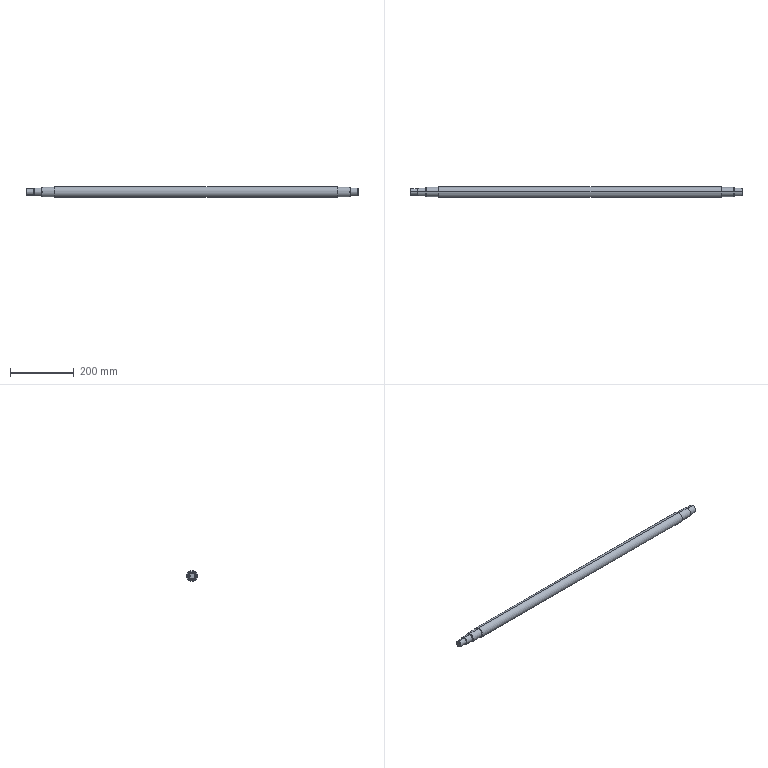Part | NX | features BREP 1 | 1 solid | 45 faces | box 1045 x 34 x 34 mm | volume 895297 mm3 | cylinder 18 | plane 17 | cone 10 | commonest cylinder face diameters 8 x4 25 x4 30 x4 6 x2 20 x2 34 x2
STEP:
#1=CARTESIAN_POINT('',(90.,0.,-17.));
#2=VERTEX_POINT('',#1);
#3=CARTESIAN_POINT('',(980.,0.,-17.));
#4=VERTEX_POINT('',#3);
#5=CARTESIAN_POINT('',(980.,0.,-17.));
#6=DIRECTION('',(-1.,0.,0.));
#7=VECTOR('',#6,1000.);
#8=LINE('',#5,#7);
#9=EDGE_CURVE('',#2,#4,#8,.F.);
#10=ORIENTED_EDGE('',*,*,#9,.T.);
#11=CARTESIAN_POINT('',(980.,0.,17.));
#12=VERTEX_POINT('',#11);
#13=CARTESIAN_POINT('',(980.,0.,0.));
#14=DIRECTION('',(-1.,0.,0.));
#15=DIRECTION('',(0.,0.,1.));
#16=AXIS2_PLACEMENT_3D('',#13,#14,#15);
#17=CIRCLE('',#16,17.);
#18=EDGE_CURVE('',#4,#12,#17,.T.);
#19=ORIENTED_EDGE('',*,*,#18,.T.);
#20=CARTESIAN_POINT('',(90.,0.,17.));
#21=VERTEX_POINT('',#20);
#22=CARTESIAN_POINT('',(980.,0.,17.));
#23=DIRECTION('',(-1.,0.,0.));
#24=VECTOR('',#23,1000.);
#25=LINE('',#22,#24);
#26=EDGE_CURVE('',#21,#12,#25,.F.);
#27=ORIENTED_EDGE('',*,*,#26,.F.);
#28=CARTESIAN_POINT('',(90.,0.,0.));
#29=DIRECTION('',(1.,0.,0.));
#30=DIRECTION('',(0.,0.,1.));
#31=AXIS2_PLACEMENT_3D('',#28,#29,#30);
#32=CIRCLE('',#31,17.);
#33=EDGE_CURVE('',#21,#2,#32,.T.);
#34=ORIENTED_EDGE('',*,*,#33,.T.);
#35=EDGE_LOOP('',(#10,#19,#27,#34));
#36=FACE_BOUND('',#35,.T.);
#37=CARTESIAN_POINT('',(980.,0.,0.));
#38=DIRECTION('',(-1.,0.,0.));
#39=DIRECTION('',(0.,0.,1.));
#40=AXIS2_PLACEMENT_3D('',#37,#38,#39);
#41=CYLINDRICAL_SURFACE('',#40,17.);
#42=ADVANCED_FACE('',(#36),#41,.T.);
#43=CARTESIAN_POINT('',(90.,0.,15.));
#44=VERTEX_POINT('',#43);
#45=CARTESIAN_POINT('',(90.,0.,-15.));
#46=VERTEX_POINT('',#45);
#47=CARTESIAN_POINT('',(90.,0.,0.));
#48=DIRECTION('',(-1.,0.,0.));
#49=DIRECTION('',(0.,0.,1.));
#50=AXIS2_PLACEMENT_3D('',#47,#48,#49);
#51=CIRCLE('',#50,15.);
#52=EDGE_CURVE('',#44,#46,#51,.T.);
#53=ORIENTED_EDGE('',*,*,#52,.F.);
#54=CARTESIAN_POINT('',(90.,0.,0.));
#55=DIRECTION('',(-1.,0.,0.));
#56=DIRECTION('',(0.,0.,1.));
#57=AXIS2_PLACEMENT_3D('',#54,#55,#56);
#58=CIRCLE('',#57,15.);
#59=EDGE_CURVE('',#46,#44,#58,.T.);
#60=ORIENTED_EDGE('',*,*,#59,.F.);
#61=EDGE_LOOP('',(#53,#60));
#62=FACE_BOUND('',#61,.T.);
#63=ORIENTED_EDGE('',*,*,#33,.F.);
#64=CARTESIAN_POINT('',(90.,0.,0.));
#65=DIRECTION('',(1.,0.,0.));
#66=DIRECTION('',(0.,0.,1.));
#67=AXIS2_PLACEMENT_3D('',#64,#65,#66);
#68=CIRCLE('',#67,17.);
#69=EDGE_CURVE('',#2,#21,#68,.T.);
#70=ORIENTED_EDGE('',*,*,#69,.F.);
#71=EDGE_LOOP('',(#63,#70));
#72=FACE_BOUND('',#71,.T.);
#73=CARTESIAN_POINT('',(90.,0.,0.));
#74=DIRECTION('',(1.,0.,0.));
#75=DIRECTION('',(0.,1.,0.));
#76=AXIS2_PLACEMENT_3D('',#73,#74,#75);
#77=PLANE('',#76);
#78=ADVANCED_FACE('',(#62,#72),#77,.F.);
#79=CARTESIAN_POINT('',(980.,0.,15.));
#80=VERTEX_POINT('',#79);
#81=CARTESIAN_POINT('',(980.,0.,-15.));
#82=VERTEX_POINT('',#81);
#83=CARTESIAN_POINT('',(980.,0.,0.));
#84=DIRECTION('',(-1.,0.,0.));
#85=DIRECTION('',(0.,0.,1.));
#86=AXIS2_PLACEMENT_3D('',#83,#84,#85);
#87=CIRCLE('',#86,15.);
#88=EDGE_CURVE('',#80,#82,#87,.T.);
#89=ORIENTED_EDGE('',*,*,#88,.T.);
#90=CARTESIAN_POINT('',(980.,0.,0.));
#91=DIRECTION('',(-1.,0.,0.));
#92=DIRECTION('',(0.,0.,1.));
#93=AXIS2_PLACEMENT_3D('',#90,#91,#92);
#94=CIRCLE('',#93,15.);
#95=EDGE_CURVE('',#82,#80,#94,.T.);
#96=ORIENTED_EDGE('',*,*,#95,.T.);
#97=EDGE_LOOP('',(#89,#96));
#98=FACE_BOUND('',#97,.T.);
#99=CARTESIAN_POINT('',(980.,0.,0.));
#100=DIRECTION('',(-1.,0.,0.));
#101=DIRECTION('',(0.,0.,1.));
#102=AXIS2_PLACEMENT_3D('',#99,#100,#101);
#103=CIRCLE('',#102,17.);
#104=EDGE_CURVE('',#12,#4,#103,.T.);
#105=ORIENTED_EDGE('',*,*,#104,.F.);
#106=ORIENTED_EDGE('',*,*,#18,.F.);
#107=EDGE_LOOP('',(#105,#106));
#108=FACE_BOUND('',#107,.T.);
#109=CARTESIAN_POINT('',(980.,0.,0.));
#110=DIRECTION('',(1.,0.,0.));
#111=DIRECTION('',(0.,1.,0.));
#112=AXIS2_PLACEMENT_3D('',#109,#110,#111);
#113=PLANE('',#112);
#114=ADVANCED_FACE('',(#98,#108),#113,.T.);
#115=CARTESIAN_POINT('',(51.,0.,-15.));
#116=VERTEX_POINT('',#115);
#117=CARTESIAN_POINT('',(90.,0.,-15.));
#118=DIRECTION('',(-1.,0.,0.));
#119=VECTOR('',#118,1000.);
#120=LINE('',#117,#119);
#121=EDGE_CURVE('',#116,#46,#120,.F.);
#122=ORIENTED_EDGE('',*,*,#121,.T.);
#123=ORIENTED_EDGE('',*,*,#59,.T.);
#124=CARTESIAN_POINT('',(51.,0.,15.));
#125=VERTEX_POINT('',#124);
#126=CARTESIAN_POINT('',(90.,0.,15.));
#127=DIRECTION('',(-1.,0.,0.));
#128=VECTOR('',#127,1000.);
#129=LINE('',#126,#128);
#130=EDGE_CURVE('',#125,#44,#129,.F.);
#131=ORIENTED_EDGE('',*,*,#130,.F.);
#132=CARTESIAN_POINT('',(51.,0.,0.));
#133=DIRECTION('',(1.,0.,0.));
#134=DIRECTION('',(0.,0.,1.));
#135=AXIS2_PLACEMENT_3D('',#132,#133,#134);
#136=CIRCLE('',#135,15.);
#137=EDGE_CURVE('',#125,#116,#136,.T.);
#138=ORIENTED_EDGE('',*,*,#137,.T.);
#139=EDGE_LOOP('',(#122,#123,#131,#138));
#140=FACE_BOUND('',#139,.T.);
#141=CARTESIAN_POINT('',(90.,0.,0.));
#142=DIRECTION('',(-1.,0.,0.));
#143=DIRECTION('',(0.,0.,1.));
#144=AXIS2_PLACEMENT_3D('',#141,#142,#143);
#145=CYLINDRICAL_SURFACE('',#144,15.);
#146=ADVANCED_FACE('',(#140),#145,.T.);
#147=CARTESIAN_POINT('',(1019.,0.,-15.));
#148=VERTEX_POINT('',#147);
#149=CARTESIAN_POINT('',(1020.,0.,-15.));
#150=DIRECTION('',(-1.,0.,0.));
#151=VECTOR('',#150,1000.);
#152=LINE('',#149,#151);
#153=EDGE_CURVE('',#82,#148,#152,.F.);
#154=ORIENTED_EDGE('',*,*,#153,.T.);
#155=CARTESIAN_POINT('',(1019.,0.,15.));
#156=VERTEX_POINT('',#155);
#157=CARTESIAN_POINT('',(1019.,0.,0.));
#158=DIRECTION('',(-1.,0.,0.));
#159=DIRECTION('',(0.,0.,1.));
#160=AXIS2_PLACEMENT_3D('',#157,#158,#159);
#161=CIRCLE('',#160,15.);
#162=EDGE_CURVE('',#148,#156,#161,.T.);
#163=ORIENTED_EDGE('',*,*,#162,.T.);
#164=CARTESIAN_POINT('',(1020.,0.,15.));
#165=DIRECTION('',(-1.,0.,0.));
#166=VECTOR('',#165,1000.);
#167=LINE('',#164,#166);
#168=EDGE_CURVE('',#80,#156,#167,.F.);
#169=ORIENTED_EDGE('',*,*,#168,.F.);
#170=ORIENTED_EDGE('',*,*,#95,.F.);
#171=EDGE_LOOP('',(#154,#163,#169,#170));
#172=FACE_BOUND('',#171,.T.);
#173=CARTESIAN_POINT('',(1020.,0.,0.));
#174=DIRECTION('',(-1.,0.,0.));
#175=DIRECTION('',(0.,0.,1.));
#176=AXIS2_PLACEMENT_3D('',#173,#174,#175);
#177=CYLINDRICAL_SURFACE('',#176,15.);
#178=ADVANCED_FACE('',(#172),#177,.T.);
#179=CARTESIAN_POINT('',(50.,0.,14.));
#180=VERTEX_POINT('',#179);
#181=CARTESIAN_POINT('',(51.,0.,15.));
#182=DIRECTION('',(0.7071,0.,0.7071));
#183=VECTOR('',#182,1000.);
#184=LINE('',#181,#183);
#185=EDGE_CURVE('',#180,#125,#184,.T.);
#186=ORIENTED_EDGE('',*,*,#185,.F.);
#187=CARTESIAN_POINT('',(50.,0.,-14.));
#188=VERTEX_POINT('',#187);
#189=CARTESIAN_POINT('',(50.,0.,0.));
#190=DIRECTION('',(1.,0.,0.));
#191=DIRECTION('',(0.,0.,-1.));
#192=AXIS2_PLACEMENT_3D('',#189,#190,#191);
#193=CIRCLE('',#192,14.);
#194=EDGE_CURVE('',#180,#188,#193,.T.);
#195=ORIENTED_EDGE('',*,*,#194,.T.);
#196=CARTESIAN_POINT('',(51.,0.,-15.));
#197=DIRECTION('',(0.7071,0.,-0.7071));
#198=VECTOR('',#197,1000.);
#199=LINE('',#196,#198);
#200=EDGE_CURVE('',#188,#116,#199,.T.);
#201=ORIENTED_EDGE('',*,*,#200,.T.);
#202=ORIENTED_EDGE('',*,*,#137,.F.);
#203=EDGE_LOOP('',(#186,#195,#201,#202));
#204=FACE_BOUND('',#203,.T.);
#205=CARTESIAN_POINT('',(51.,0.,0.));
#206=DIRECTION('',(1.,0.,0.));
#207=DIRECTION('',(0.,0.,-1.));
#208=AXIS2_PLACEMENT_3D('',#205,#206,#207);
#209=CONICAL_SURFACE('',#208,15.,0.7854);
#210=ADVANCED_FACE('',(#204),#209,.T.);
#211=CARTESIAN_POINT('',(64.,11.7,-4.));
#212=VERTEX_POINT('',#211);
#213=CARTESIAN_POINT('',(64.,11.7,4.));
#214=VERTEX_POINT('',#213);
#215=CARTESIAN_POINT('',(64.,11.7,0.));
#216=DIRECTION('',(0.,1.,0.));
#217=DIRECTION('',(0.,0.,1.));
#218=AXIS2_PLACEMENT_3D('',#215,#216,#217);
#219=CIRCLE('',#218,4.);
#220=EDGE_CURVE('',#212,#214,#219,.T.);
#221=ORIENTED_EDGE('',*,*,#220,.F.);
#222=CARTESIAN_POINT('',(64.,14.457,-4.));
#223=VERTEX_POINT('',#222);
#224=CARTESIAN_POINT('',(64.,11.7,-4.));
#225=DIRECTION('',(0.,-1.,0.));
#226=VECTOR('',#225,1000.);
#227=LINE('',#224,#226);
#228=EDGE_CURVE('',#223,#212,#227,.T.);
#229=ORIENTED_EDGE('',*,*,#228,.F.);
#230=CARTESIAN_POINT('',(64.,14.457,4.));
#231=VERTEX_POINT('',#230);
#232=CARTESIAN_POINT('',(64.,14.457,-4.));
#233=CARTESIAN_POINT('',(63.752,14.457,-4.));
#234=CARTESIAN_POINT('',(63.255,14.469,-3.961));
#235=CARTESIAN_POINT('',(62.553,14.526,-3.742));
#236=CARTESIAN_POINT('',(62.143,14.574,-3.552));
#237=CARTESIAN_POINT('',(61.735,14.632,-3.303));
#238=CARTESIAN_POINT('',(61.55,14.662,-3.168));
#239=CARTESIAN_POINT('',(61.156,14.732,-2.831));
#240=CARTESIAN_POINT('',(60.849,14.796,-2.471));
#241=CARTESIAN_POINT('',(60.688,14.831,-2.253));
#242=CARTESIAN_POINT('',(60.447,14.886,-1.854));
#243=CARTESIAN_POINT('',(60.255,14.934,-1.44));
#244=CARTESIAN_POINT('',(60.039,14.989,-0.7446));
#245=CARTESIAN_POINT('',(59.98,15.006,0.003989));
#246=CARTESIAN_POINT('',(60.041,14.988,0.7508));
#247=CARTESIAN_POINT('',(60.257,14.933,1.444));
#248=CARTESIAN_POINT('',(60.45,14.886,1.86));
#249=CARTESIAN_POINT('',(60.691,14.83,2.257));
#250=CARTESIAN_POINT('',(60.847,14.796,2.468));
#251=CARTESIAN_POINT('',(61.158,14.732,2.833));
#252=CARTESIAN_POINT('',(61.552,14.662,3.17));
#253=CARTESIAN_POINT('',(61.74,14.631,3.307));
#254=CARTESIAN_POINT('',(62.146,14.574,3.553));
#255=CARTESIAN_POINT('',(62.553,14.526,3.742));
#256=CARTESIAN_POINT('',(63.256,14.469,3.961));
#257=CARTESIAN_POINT('',(63.753,14.457,4.));
#258=CARTESIAN_POINT('',(64.,14.457,4.));
#259=B_SPLINE_CURVE_WITH_KNOTS('',3,(#232,#233,#234,#235,#236,#237,#238,#239,#240,#241,#242,#243,#244,#245,#246,#247,#248,#249,#250,#251,#252,#253,#254,#255,#256,#257,#258),.UNSPECIFIED.,.F.,.F.,(4,1,1,1,1,1,1,1,1,1,1,1,1,1,1,1,1,1,1,1,1,1,1,1,4),(0.,0.0625,0.125,0.1562,0.1875,0.2188,0.25,0.2812,0.3125,0.3438,0.375,0.4375,0.5,0.5625,0.625,0.6562,0.6875,0.7188,0.75,0.7812,0.8125,0.8438,0.875,0.9375,1.),.UNSPECIFIED.);
#260=EDGE_CURVE('',#231,#223,#259,.F.);
#261=ORIENTED_EDGE('',*,*,#260,.F.);
#262=CARTESIAN_POINT('',(64.,11.7,4.));
#263=DIRECTION('',(0.,1.,0.));
#264=VECTOR('',#263,1000.);
#265=LINE('',#262,#264);
#266=EDGE_CURVE('',#214,#231,#265,.T.);
#267=ORIENTED_EDGE('',*,*,#266,.F.);
#268=EDGE_LOOP('',(#221,#229,#261,#267));
#269=FACE_BOUND('',#268,.T.);
#270=CARTESIAN_POINT('',(64.,11.7,0.));
#271=DIRECTION('',(0.,1.,0.));
#272=DIRECTION('',(0.,0.,1.));
#273=AXIS2_PLACEMENT_3D('',#270,#271,#272);
#274=CYLINDRICAL_SURFACE('',#273,4.);
#275=ADVANCED_FACE('',(#269),#274,.F.);
#276=CARTESIAN_POINT('',(81.,11.7,4.));
#277=VERTEX_POINT('',#276);
#278=CARTESIAN_POINT('',(64.,11.7,4.));
#279=DIRECTION('',(1.,0.,0.));
#280=VECTOR('',#279,1000.);
#281=LINE('',#278,#280);
#282=EDGE_CURVE('',#214,#277,#281,.T.);
#283=ORIENTED_EDGE('',*,*,#282,.F.);
#284=ORIENTED_EDGE('',*,*,#266,.T.);
#285=CARTESIAN_POINT('',(81.,14.457,4.));
#286=VERTEX_POINT('',#285);
#287=CARTESIAN_POINT('',(90.,14.457,4.));
#288=DIRECTION('',(-1.,0.,0.));
#289=VECTOR('',#288,1000.);
#290=LINE('',#287,#289);
#291=EDGE_CURVE('',#286,#231,#290,.T.);
#292=ORIENTED_EDGE('',*,*,#291,.F.);
#293=CARTESIAN_POINT('',(81.,11.7,4.));
#294=DIRECTION('',(0.,1.,0.));
#295=VECTOR('',#294,1000.);
#296=LINE('',#293,#295);
#297=EDGE_CURVE('',#277,#286,#296,.T.);
#298=ORIENTED_EDGE('',*,*,#297,.F.);
#299=EDGE_LOOP('',(#283,#284,#292,#298));
#300=FACE_BOUND('',#299,.T.);
#301=CARTESIAN_POINT('',(64.,11.7,4.));
#302=DIRECTION('',(0.,0.,1.));
#303=DIRECTION('',(1.,0.,0.));
#304=AXIS2_PLACEMENT_3D('',#301,#302,#303);
#305=PLANE('',#304);
#306=ADVANCED_FACE('',(#300),#305,.F.);
#307=CARTESIAN_POINT('',(81.,11.7,-4.));
#308=VERTEX_POINT('',#307);
#309=CARTESIAN_POINT('',(81.,11.7,0.));
#310=DIRECTION('',(0.,1.,0.));
#311=DIRECTION('',(0.,0.,1.));
#312=AXIS2_PLACEMENT_3D('',#309,#310,#311);
#313=CIRCLE('',#312,4.);
#314=EDGE_CURVE('',#277,#308,#313,.T.);
#315=ORIENTED_EDGE('',*,*,#314,.F.);
#316=ORIENTED_EDGE('',*,*,#297,.T.);
#317=CARTESIAN_POINT('',(81.,14.457,-4.));
#318=VERTEX_POINT('',#317);
#319=CARTESIAN_POINT('',(81.,14.457,4.));
#320=CARTESIAN_POINT('',(81.248,14.457,4.));
#321=CARTESIAN_POINT('',(81.745,14.469,3.961));
#322=CARTESIAN_POINT('',(82.447,14.526,3.742));
#323=CARTESIAN_POINT('',(82.857,14.574,3.552));
#324=CARTESIAN_POINT('',(83.265,14.632,3.303));
#325=CARTESIAN_POINT('',(83.45,14.662,3.168));
#326=CARTESIAN_POINT('',(83.844,14.732,2.831));
#327=CARTESIAN_POINT('',(84.151,14.796,2.471));
#328=CARTESIAN_POINT('',(84.312,14.831,2.253));
#329=CARTESIAN_POINT('',(84.553,14.886,1.854));
#330=CARTESIAN_POINT('',(84.745,14.934,1.44));
#331=CARTESIAN_POINT('',(84.961,14.989,0.7446));
#332=CARTESIAN_POINT('',(85.02,15.006,-0.003989));
#333=CARTESIAN_POINT('',(84.959,14.988,-0.7508));
#334=CARTESIAN_POINT('',(84.743,14.933,-1.444));
#335=CARTESIAN_POINT('',(84.55,14.886,-1.86));
#336=CARTESIAN_POINT('',(84.309,14.83,-2.257));
#337=CARTESIAN_POINT('',(84.153,14.796,-2.468));
#338=CARTESIAN_POINT('',(83.842,14.732,-2.833));
#339=CARTESIAN_POINT('',(83.448,14.662,-3.17));
#340=CARTESIAN_POINT('',(83.26,14.631,-3.307));
#341=CARTESIAN_POINT('',(82.854,14.574,-3.553));
#342=CARTESIAN_POINT('',(82.447,14.526,-3.742));
#343=CARTESIAN_POINT('',(81.744,14.469,-3.961));
#344=CARTESIAN_POINT('',(81.247,14.457,-4.));
#345=CARTESIAN_POINT('',(81.,14.457,-4.));
#346=B_SPLINE_CURVE_WITH_KNOTS('',3,(#319,#320,#321,#322,#323,#324,#325,#326,#327,#328,#329,#330,#331,#332,#333,#334,#335,#336,#337,#338,#339,#340,#341,#342,#343,#344,#345),.UNSPECIFIED.,.F.,.F.,(4,1,1,1,1,1,1,1,1,1,1,1,1,1,1,1,1,1,1,1,1,1,1,1,4),(0.,0.0625,0.125,0.1562,0.1875,0.2188,0.25,0.2812,0.3125,0.3438,0.375,0.4375,0.5,0.5625,0.625,0.6562,0.6875,0.7188,0.75,0.7812,0.8125,0.8438,0.875,0.9375,1.),.UNSPECIFIED.);
#347=EDGE_CURVE('',#318,#286,#346,.F.);
#348=ORIENTED_EDGE('',*,*,#347,.F.);
#349=CARTESIAN_POINT('',(81.,11.7,-4.));
#350=DIRECTION('',(0.,1.,0.));
#351=VECTOR('',#350,1000.);
#352=LINE('',#349,#351);
#353=EDGE_CURVE('',#308,#318,#352,.T.);
#354=ORIENTED_EDGE('',*,*,#353,.F.);
#355=EDGE_LOOP('',(#315,#316,#348,#354));
#356=FACE_BOUND('',#355,.T.);
#357=CARTESIAN_POINT('',(81.,11.7,0.));
#358=DIRECTION('',(0.,1.,0.));
#359=DIRECTION('',(0.,0.,1.));
#360=AXIS2_PLACEMENT_3D('',#357,#358,#359);
#361=CYLINDRICAL_SURFACE('',#360,4.);
#362=ADVANCED_FACE('',(#356),#361,.F.);
#363=CARTESIAN_POINT('',(64.,11.7,-4.));
#364=DIRECTION('',(-1.,0.,0.));
#365=VECTOR('',#364,1000.);
#366=LINE('',#363,#365);
#367=EDGE_CURVE('',#308,#212,#366,.T.);
#368=ORIENTED_EDGE('',*,*,#367,.F.);
#369=ORIENTED_EDGE('',*,*,#353,.T.);
#370=CARTESIAN_POINT('',(90.,14.457,-4.));
#371=DIRECTION('',(1.,0.,0.));
#372=VECTOR('',#371,1000.);
#373=LINE('',#370,#372);
#374=EDGE_CURVE('',#223,#318,#373,.T.);
#375=ORIENTED_EDGE('',*,*,#374,.F.);
#376=ORIENTED_EDGE('',*,*,#228,.T.);
#377=EDGE_LOOP('',(#368,#369,#375,#376));
#378=FACE_BOUND('',#377,.T.);
#379=CARTESIAN_POINT('',(64.,11.7,-4.));
#380=DIRECTION('',(0.,0.,-1.));
#381=DIRECTION('',(-1.,0.,0.));
#382=AXIS2_PLACEMENT_3D('',#379,#380,#381);
#383=PLANE('',#382);
#384=ADVANCED_FACE('',(#378),#383,.F.);
#385=CARTESIAN_POINT('',(1020.,0.,-14.));
#386=VERTEX_POINT('',#385);
#387=CARTESIAN_POINT('',(1019.,0.,-15.));
#388=DIRECTION('',(-0.7071,0.,-0.7071));
#389=VECTOR('',#388,1000.);
#390=LINE('',#387,#389);
#391=EDGE_CURVE('',#148,#386,#390,.F.);
#392=ORIENTED_EDGE('',*,*,#391,.T.);
#393=CARTESIAN_POINT('',(1020.,0.,14.));
#394=VERTEX_POINT('',#393);
#395=CARTESIAN_POINT('',(1020.,0.,0.));
#396=DIRECTION('',(-1.,0.,0.));
#397=DIRECTION('',(0.,0.,1.));
#398=AXIS2_PLACEMENT_3D('',#395,#396,#397);
#399=CIRCLE('',#398,14.);
#400=EDGE_CURVE('',#386,#394,#399,.T.);
#401=ORIENTED_EDGE('',*,*,#400,.T.);
#402=CARTESIAN_POINT('',(1019.,0.,15.));
#403=DIRECTION('',(-0.7071,0.,0.7071));
#404=VECTOR('',#403,1000.);
#405=LINE('',#402,#404);
#406=EDGE_CURVE('',#156,#394,#405,.F.);
#407=ORIENTED_EDGE('',*,*,#406,.F.);
#408=ORIENTED_EDGE('',*,*,#162,.F.);
#409=EDGE_LOOP('',(#392,#401,#407,#408));
#410=FACE_BOUND('',#409,.T.);
#411=CARTESIAN_POINT('',(1019.,0.,0.));
#412=DIRECTION('',(-1.,0.,0.));
#413=DIRECTION('',(0.,0.,1.));
#414=AXIS2_PLACEMENT_3D('',#411,#412,#413);
#415=CONICAL_SURFACE('',#414,15.,0.7854);
#416=ADVANCED_FACE('',(#410),#415,.T.);
#417=CARTESIAN_POINT('',(50.,0.,12.5));
#418=VERTEX_POINT('',#417);
#419=CARTESIAN_POINT('',(50.,0.,-12.5));
#420=VERTEX_POINT('',#419);
#421=CARTESIAN_POINT('',(50.,0.,0.));
#422=DIRECTION('',(-1.,0.,0.));
#423=DIRECTION('',(0.,0.,1.));
#424=AXIS2_PLACEMENT_3D('',#421,#422,#423);
#425=CIRCLE('',#424,12.5);
#426=EDGE_CURVE('',#418,#420,#425,.T.);
#427=ORIENTED_EDGE('',*,*,#426,.F.);
#428=CARTESIAN_POINT('',(50.,0.,0.));
#429=DIRECTION('',(-1.,0.,0.));
#430=DIRECTION('',(0.,0.,1.));
#431=AXIS2_PLACEMENT_3D('',#428,#429,#430);
#432=CIRCLE('',#431,12.5);
#433=EDGE_CURVE('',#420,#418,#432,.T.);
#434=ORIENTED_EDGE('',*,*,#433,.F.);
#435=EDGE_LOOP('',(#427,#434));
#436=FACE_BOUND('',#435,.T.);
#437=CARTESIAN_POINT('',(50.,0.,0.));
#438=DIRECTION('',(1.,0.,0.));
#439=DIRECTION('',(0.,0.,-1.));
#440=AXIS2_PLACEMENT_3D('',#437,#438,#439);
#441=CIRCLE('',#440,14.);
#442=EDGE_CURVE('',#188,#180,#441,.T.);
#443=ORIENTED_EDGE('',*,*,#442,.F.);
#444=ORIENTED_EDGE('',*,*,#194,.F.);
#445=EDGE_LOOP('',(#443,#444));
#446=FACE_BOUND('',#445,.T.);
#447=CARTESIAN_POINT('',(50.,0.,0.));
#448=DIRECTION('',(1.,0.,0.));
#449=DIRECTION('',(0.,1.,0.));
#450=AXIS2_PLACEMENT_3D('',#447,#448,#449);
#451=PLANE('',#450);
#452=ADVANCED_FACE('',(#436,#446),#451,.F.);
#453=ORIENTED_EDGE('',*,*,#282,.T.);
#454=ORIENTED_EDGE('',*,*,#314,.T.);
#455=ORIENTED_EDGE('',*,*,#367,.T.);
#456=ORIENTED_EDGE('',*,*,#220,.T.);
#457=EDGE_LOOP('',(#453,#454,#455,#456));
#458=FACE_BOUND('',#457,.T.);
#459=CARTESIAN_POINT('',(64.,11.7,0.));
#460=DIRECTION('',(0.,-1.,0.));
#461=DIRECTION('',(0.,0.,-1.));
#462=AXIS2_PLACEMENT_3D('',#459,#460,#461);
#463=PLANE('',#462);
#464=ADVANCED_FACE('',(#458),#463,.F.);
#465=CARTESIAN_POINT('',(1020.,0.,12.5));
#466=VERTEX_POINT('',#465);
#467=CARTESIAN_POINT('',(1020.,0.,-12.5));
#468=VERTEX_POINT('',#467);
#469=CARTESIAN_POINT('',(1020.,0.,0.));
#470=DIRECTION('',(-1.,0.,0.));
#471=DIRECTION('',(0.,0.,1.));
#472=AXIS2_PLACEMENT_3D('',#469,#470,#471);
#473=CIRCLE('',#472,12.5);
#474=EDGE_CURVE('',#466,#468,#473,.T.);
#475=ORIENTED_EDGE('',*,*,#474,.T.);
#476=CARTESIAN_POINT('',(1020.,0.,0.));
#477=DIRECTION('',(-1.,0.,0.));
#478=DIRECTION('',(0.,0.,1.));
#479=AXIS2_PLACEMENT_3D('',#476,#477,#478);
#480=CIRCLE('',#479,12.5);
#481=EDGE_CURVE('',#468,#466,#480,.T.);
#482=ORIENTED_EDGE('',*,*,#481,.T.);
#483=EDGE_LOOP('',(#475,#482));
#484=FACE_BOUND('',#483,.T.);
#485=CARTESIAN_POINT('',(1020.,0.,0.));
#486=DIRECTION('',(-1.,0.,0.));
#487=DIRECTION('',(0.,0.,1.));
#488=AXIS2_PLACEMENT_3D('',#485,#486,#487);
#489=CIRCLE('',#488,14.);
#490=EDGE_CURVE('',#394,#386,#489,.T.);
#491=ORIENTED_EDGE('',*,*,#490,.F.);
#492=ORIENTED_EDGE('',*,*,#400,.F.);
#493=EDGE_LOOP('',(#491,#492));
#494=FACE_BOUND('',#493,.T.);
#495=CARTESIAN_POINT('',(1020.,0.,0.));
#496=DIRECTION('',(1.,0.,0.));
#497=DIRECTION('',(0.,1.,0.));
#498=AXIS2_PLACEMENT_3D('',#495,#496,#497);
#499=PLANE('',#498);
#500=ADVANCED_FACE('',(#484,#494),#499,.T.);
#501=CARTESIAN_POINT('',(26.,0.,-12.5));
#502=VERTEX_POINT('',#501);
#503=CARTESIAN_POINT('',(50.,0.,-12.5));
#504=DIRECTION('',(-1.,0.,0.));
#505=VECTOR('',#504,1000.);
#506=LINE('',#503,#505);
#507=EDGE_CURVE('',#502,#420,#506,.F.);
#508=ORIENTED_EDGE('',*,*,#507,.T.);
#509=ORIENTED_EDGE('',*,*,#433,.T.);
#510=CARTESIAN_POINT('',(26.,0.,12.5));
#511=VERTEX_POINT('',#510);
#512=CARTESIAN_POINT('',(50.,0.,12.5));
#513=DIRECTION('',(-1.,0.,0.));
#514=VECTOR('',#513,1000.);
#515=LINE('',#512,#514);
#516=EDGE_CURVE('',#511,#418,#515,.F.);
#517=ORIENTED_EDGE('',*,*,#516,.F.);
#518=CARTESIAN_POINT('',(26.,0.,0.));
#519=DIRECTION('',(1.,0.,0.));
#520=DIRECTION('',(0.,0.,1.));
#521=AXIS2_PLACEMENT_3D('',#518,#519,#520);
#522=CIRCLE('',#521,12.5);
#523=EDGE_CURVE('',#511,#502,#522,.T.);
#524=ORIENTED_EDGE('',*,*,#523,.T.);
#525=EDGE_LOOP('',(#508,#509,#517,#524));
#526=FACE_BOUND('',#525,.T.);
#527=CARTESIAN_POINT('',(50.,0.,0.));
#528=DIRECTION('',(-1.,0.,0.));
#529=DIRECTION('',(0.,0.,1.));
#530=AXIS2_PLACEMENT_3D('',#527,#528,#529);
#531=CYLINDRICAL_SURFACE('',#530,12.5);
#532=ADVANCED_FACE('',(#526),#531,.T.);
#533=CARTESIAN_POINT('',(1044.,0.,-12.5));
#534=VERTEX_POINT('',#533);
#535=CARTESIAN_POINT('',(1045.,0.,-12.5));
#536=DIRECTION('',(-1.,0.,0.));
#537=VECTOR('',#536,1000.);
#538=LINE('',#535,#537);
#539=EDGE_CURVE('',#468,#534,#538,.F.);
#540=ORIENTED_EDGE('',*,*,#539,.T.);
#541=CARTESIAN_POINT('',(1044.,0.,12.5));
#542=VERTEX_POINT('',#541);
#543=CARTESIAN_POINT('',(1044.,0.,0.));
#544=DIRECTION('',(-1.,0.,0.));
#545=DIRECTION('',(0.,0.,1.));
#546=AXIS2_PLACEMENT_3D('',#543,#544,#545);
#547=CIRCLE('',#546,12.5);
#548=EDGE_CURVE('',#534,#542,#547,.T.);
#549=ORIENTED_EDGE('',*,*,#548,.T.);
#550=CARTESIAN_POINT('',(1045.,0.,12.5));
#551=DIRECTION('',(-1.,0.,0.));
#552=VECTOR('',#551,1000.);
#553=LINE('',#550,#552);
#554=EDGE_CURVE('',#466,#542,#553,.F.);
#555=ORIENTED_EDGE('',*,*,#554,.F.);
#556=ORIENTED_EDGE('',*,*,#481,.F.);
#557=EDGE_LOOP('',(#540,#549,#555,#556));
#558=FACE_BOUND('',#557,.T.);
#559=CARTESIAN_POINT('',(1045.,0.,0.));
#560=DIRECTION('',(-1.,0.,0.));
#561=DIRECTION('',(0.,0.,1.));
#562=AXIS2_PLACEMENT_3D('',#559,#560,#561);
#563=CYLINDRICAL_SURFACE('',#562,12.5);
#564=ADVANCED_FACE('',(#558),#563,.T.);
#565=CARTESIAN_POINT('',(25.,0.,11.5));
#566=VERTEX_POINT('',#565);
#567=CARTESIAN_POINT('',(26.,0.,12.5));
#568=DIRECTION('',(0.7071,0.,0.7071));
#569=VECTOR('',#568,1000.);
#570=LINE('',#567,#569);
#571=EDGE_CURVE('',#566,#511,#570,.T.);
#572=ORIENTED_EDGE('',*,*,#571,.F.);
#573=CARTESIAN_POINT('',(25.,0.,-11.5));
#574=VERTEX_POINT('',#573);
#575=CARTESIAN_POINT('',(25.,0.,0.));
#576=DIRECTION('',(1.,0.,0.));
#577=DIRECTION('',(0.,0.,-1.));
#578=AXIS2_PLACEMENT_3D('',#575,#576,#577);
#579=CIRCLE('',#578,11.5);
#580=EDGE_CURVE('',#566,#574,#579,.T.);
#581=ORIENTED_EDGE('',*,*,#580,.T.);
#582=CARTESIAN_POINT('',(26.,0.,-12.5));
#583=DIRECTION('',(0.7071,0.,-0.7071));
#584=VECTOR('',#583,1000.);
#585=LINE('',#582,#584);
#586=EDGE_CURVE('',#574,#502,#585,.T.);
#587=ORIENTED_EDGE('',*,*,#586,.T.);
#588=ORIENTED_EDGE('',*,*,#523,.F.);
#589=EDGE_LOOP('',(#572,#581,#587,#588));
#590=FACE_BOUND('',#589,.T.);
#591=CARTESIAN_POINT('',(26.,0.,0.));
#592=DIRECTION('',(1.,0.,0.));
#593=DIRECTION('',(0.,0.,-1.));
#594=AXIS2_PLACEMENT_3D('',#591,#592,#593);
#595=CONICAL_SURFACE('',#594,12.5,0.7854);
#596=ADVANCED_FACE('',(#590),#595,.T.);
#597=CARTESIAN_POINT('',(1045.,0.,-11.5));
#598=VERTEX_POINT('',#597);
#599=CARTESIAN_POINT('',(1044.,0.,-12.5));
#600=DIRECTION('',(-0.7071,0.,-0.7071));
#601=VECTOR('',#600,1000.);
#602=LINE('',#599,#601);
#603=EDGE_CURVE('',#534,#598,#602,.F.);
#604=ORIENTED_EDGE('',*,*,#603,.T.);
#605=CARTESIAN_POINT('',(1045.,0.,11.5));
#606=VERTEX_POINT('',#605);
#607=CARTESIAN_POINT('',(1045.,0.,0.));
#608=DIRECTION('',(-1.,0.,0.));
#609=DIRECTION('',(0.,0.,1.));
#610=AXIS2_PLACEMENT_3D('',#607,#608,#609);
#611=CIRCLE('',#610,11.5);
#612=EDGE_CURVE('',#598,#606,#611,.T.);
#613=ORIENTED_EDGE('',*,*,#612,.T.);
#614=CARTESIAN_POINT('',(1044.,0.,12.5));
#615=DIRECTION('',(-0.7071,0.,0.7071));
#616=VECTOR('',#615,1000.);
#617=LINE('',#614,#616);
#618=EDGE_CURVE('',#542,#606,#617,.F.);
#619=ORIENTED_EDGE('',*,*,#618,.F.);
#620=ORIENTED_EDGE('',*,*,#548,.F.);
#621=EDGE_LOOP('',(#604,#613,#619,#620));
#622=FACE_BOUND('',#621,.T.);
#623=CARTESIAN_POINT('',(1044.,0.,0.));
#624=DIRECTION('',(-1.,0.,0.));
#625=DIRECTION('',(0.,0.,1.));
#626=AXIS2_PLACEMENT_3D('',#623,#624,#625);
#627=CONICAL_SURFACE('',#626,12.5,0.7854);
#628=ADVANCED_FACE('',(#622),#627,.T.);
#629=CARTESIAN_POINT('',(25.,0.,10.));
#630=VERTEX_POINT('',#629);
#631=CARTESIAN_POINT('',(25.,0.,-10.));
#632=VERTEX_POINT('',#631);
#633=CARTESIAN_POINT('',(25.,0.,0.));
#634=DIRECTION('',(-1.,0.,0.));
#635=DIRECTION('',(0.,0.,1.));
#636=AXIS2_PLACEMENT_3D('',#633,#634,#635);
#637=CIRCLE('',#636,10.);
#638=EDGE_CURVE('',#630,#632,#637,.T.);
#639=ORIENTED_EDGE('',*,*,#638,.F.);
#640=CARTESIAN_POINT('',(25.,0.,0.));
#641=DIRECTION('',(-1.,0.,0.));
#642=DIRECTION('',(0.,0.,1.));
#643=AXIS2_PLACEMENT_3D('',#640,#641,#642);
#644=CIRCLE('',#643,10.);
#645=EDGE_CURVE('',#632,#630,#644,.T.);
#646=ORIENTED_EDGE('',*,*,#645,.F.);
#647=EDGE_LOOP('',(#639,#646));
#648=FACE_BOUND('',#647,.T.);
#649=CARTESIAN_POINT('',(25.,0.,0.));
#650=DIRECTION('',(1.,0.,0.));
#651=DIRECTION('',(0.,0.,-1.));
#652=AXIS2_PLACEMENT_3D('',#649,#650,#651);
#653=CIRCLE('',#652,11.5);
#654=EDGE_CURVE('',#574,#566,#653,.T.);
#655=ORIENTED_EDGE('',*,*,#654,.F.);
#656=ORIENTED_EDGE('',*,*,#580,.F.);
#657=EDGE_LOOP('',(#655,#656));
#658=FACE_BOUND('',#657,.T.);
#659=CARTESIAN_POINT('',(25.,0.,0.));
#660=DIRECTION('',(1.,0.,0.));
#661=DIRECTION('',(0.,1.,0.));
#662=AXIS2_PLACEMENT_3D('',#659,#660,#661);
#663=PLANE('',#662);
#664=ADVANCED_FACE('',(#648,#658),#663,.F.);
#665=CARTESIAN_POINT('',(1045.,0.,0.));
#666=DIRECTION('',(-1.,0.,0.));
#667=DIRECTION('',(0.,0.,1.));
#668=AXIS2_PLACEMENT_3D('',#665,#666,#667);
#669=CIRCLE('',#668,11.5);
#670=EDGE_CURVE('',#606,#598,#669,.T.);
#671=ORIENTED_EDGE('',*,*,#670,.F.);
#672=ORIENTED_EDGE('',*,*,#612,.F.);
#673=EDGE_LOOP('',(#671,#672));
#674=FACE_BOUND('',#673,.T.);
#675=CARTESIAN_POINT('',(1045.,0.,0.));
#676=DIRECTION('',(1.,0.,0.));
#677=DIRECTION('',(0.,1.,0.));
#678=AXIS2_PLACEMENT_3D('',#675,#676,#677);
#679=PLANE('',#678);
#680=ADVANCED_FACE('',(#674),#679,.T.);
#681=CARTESIAN_POINT('',(1.,0.,-10.));
#682=VERTEX_POINT('',#681);
#683=CARTESIAN_POINT('',(25.,0.,-10.));
#684=DIRECTION('',(-1.,0.,0.));
#685=VECTOR('',#684,1000.);
#686=LINE('',#683,#685);
#687=EDGE_CURVE('',#682,#632,#686,.F.);
#688=ORIENTED_EDGE('',*,*,#687,.T.);
#689=ORIENTED_EDGE('',*,*,#645,.T.);
#690=CARTESIAN_POINT('',(1.,0.,10.));
#691=VERTEX_POINT('',#690);
#692=CARTESIAN_POINT('',(25.,0.,10.));
#693=DIRECTION('',(-1.,0.,0.));
#694=VECTOR('',#693,1000.);
#695=LINE('',#692,#694);
#696=EDGE_CURVE('',#691,#630,#695,.F.);
#697=ORIENTED_EDGE('',*,*,#696,.F.);
#698=CARTESIAN_POINT('',(1.,0.,0.));
#699=DIRECTION('',(1.,0.,0.));
#700=DIRECTION('',(0.,0.,1.));
#701=AXIS2_PLACEMENT_3D('',#698,#699,#700);
#702=CIRCLE('',#701,10.);
#703=EDGE_CURVE('',#691,#682,#702,.T.);
#704=ORIENTED_EDGE('',*,*,#703,.T.);
#705=EDGE_LOOP('',(#688,#689,#697,#704));
#706=FACE_BOUND('',#705,.T.);
#707=CARTESIAN_POINT('',(25.,0.,0.));
#708=DIRECTION('',(-1.,0.,0.));
#709=DIRECTION('',(0.,0.,1.));
#710=AXIS2_PLACEMENT_3D('',#707,#708,#709);
#711=CYLINDRICAL_SURFACE('',#710,10.);
#712=ADVANCED_FACE('',(#706),#711,.T.);
#713=CARTESIAN_POINT('',(0.,0.,9.));
#714=VERTEX_POINT('',#713);
#715=CARTESIAN_POINT('',(1.,0.,10.));
#716=DIRECTION('',(0.7071,0.,0.7071));
#717=VECTOR('',#716,1000.);
#718=LINE('',#715,#717);
#719=EDGE_CURVE('',#714,#691,#718,.T.);
#720=ORIENTED_EDGE('',*,*,#719,.F.);
#721=CARTESIAN_POINT('',(0.,0.,-9.));
#722=VERTEX_POINT('',#721);
#723=CARTESIAN_POINT('',(0.,0.,0.));
#724=DIRECTION('',(1.,0.,0.));
#725=DIRECTION('',(0.,0.,-1.));
#726=AXIS2_PLACEMENT_3D('',#723,#724,#725);
#727=CIRCLE('',#726,9.);
#728=EDGE_CURVE('',#714,#722,#727,.T.);
#729=ORIENTED_EDGE('',*,*,#728,.T.);
#730=CARTESIAN_POINT('',(1.,0.,-10.));
#731=DIRECTION('',(0.7071,0.,-0.7071));
#732=VECTOR('',#731,1000.);
#733=LINE('',#730,#732);
#734=EDGE_CURVE('',#722,#682,#733,.T.);
#735=ORIENTED_EDGE('',*,*,#734,.T.);
#736=ORIENTED_EDGE('',*,*,#703,.F.);
#737=EDGE_LOOP('',(#720,#729,#735,#736));
#738=FACE_BOUND('',#737,.T.);
#739=CARTESIAN_POINT('',(1.,0.,0.));
#740=DIRECTION('',(1.,0.,0.));
#741=DIRECTION('',(0.,0.,-1.));
#742=AXIS2_PLACEMENT_3D('',#739,#740,#741);
#743=CONICAL_SURFACE('',#742,10.,0.7854);
#744=ADVANCED_FACE('',(#738),#743,.T.);
#745=CARTESIAN_POINT('',(5.5,5.9,-3.));
#746=VERTEX_POINT('',#745);
#747=CARTESIAN_POINT('',(5.5,5.9,3.));
#748=VERTEX_POINT('',#747);
#749=CARTESIAN_POINT('',(5.5,5.9,0.));
#750=DIRECTION('',(0.,1.,0.));
#751=DIRECTION('',(0.,0.,1.));
#752=AXIS2_PLACEMENT_3D('',#749,#750,#751);
#753=CIRCLE('',#752,3.);
#754=EDGE_CURVE('',#746,#748,#753,.T.);
#755=ORIENTED_EDGE('',*,*,#754,.F.);
#756=CARTESIAN_POINT('',(5.5,9.539,-3.));
#757=VERTEX_POINT('',#756);
#758=CARTESIAN_POINT('',(5.5,5.9,-3.));
#759=DIRECTION('',(0.,-1.,0.));
#760=VECTOR('',#759,1000.);
#761=LINE('',#758,#760);
#762=EDGE_CURVE('',#757,#746,#761,.T.);
#763=ORIENTED_EDGE('',*,*,#762,.F.);
#764=CARTESIAN_POINT('',(5.5,9.539,3.));
#765=VERTEX_POINT('',#764);
#766=CARTESIAN_POINT('',(5.5,9.539,-3.));
#767=CARTESIAN_POINT('',(5.314,9.539,-3.));
#768=CARTESIAN_POINT('',(4.946,9.549,-2.974));
#769=CARTESIAN_POINT('',(4.292,9.611,-2.762));
#770=CARTESIAN_POINT('',(3.963,9.66,-2.595));
#771=CARTESIAN_POINT('',(3.347,9.774,-2.143));
#772=CARTESIAN_POINT('',(2.918,9.88,-1.556));
#773=CARTESIAN_POINT('',(2.732,9.933,-1.196));
#774=CARTESIAN_POINT('',(2.527,9.991,-0.5564));
#775=CARTESIAN_POINT('',(2.486,10.005,0.003339));
#776=CARTESIAN_POINT('',(2.528,9.991,0.5609));
#777=CARTESIAN_POINT('',(2.734,9.932,1.2));
#778=CARTESIAN_POINT('',(2.92,9.88,1.558));
#779=CARTESIAN_POINT('',(3.347,9.773,2.144));
#780=CARTESIAN_POINT('',(3.964,9.66,2.595));
#781=CARTESIAN_POINT('',(4.294,9.611,2.762));
#782=CARTESIAN_POINT('',(4.946,9.549,2.974));
#783=CARTESIAN_POINT('',(5.314,9.539,3.));
#784=CARTESIAN_POINT('',(5.5,9.539,3.));
#785=B_SPLINE_CURVE_WITH_KNOTS('',3,(#766,#767,#768,#769,#770,#771,#772,#773,#774,#775,#776,#777,#778,#779,#780,#781,#782,#783,#784),.UNSPECIFIED.,.F.,.F.,(4,1,1,1,1,1,1,1,1,1,1,1,1,1,1,1,4),(0.,0.0625,0.125,0.1875,0.25,0.3125,0.375,0.4375,0.5,0.5625,0.625,0.6875,0.75,0.8125,0.875,0.9375,1.),.UNSPECIFIED.);
#786=EDGE_CURVE('',#765,#757,#785,.F.);
#787=ORIENTED_EDGE('',*,*,#786,.F.);
#788=CARTESIAN_POINT('',(5.5,5.9,3.));
#789=DIRECTION('',(0.,1.,0.));
#790=VECTOR('',#789,1000.);
#791=LINE('',#788,#790);
#792=EDGE_CURVE('',#748,#765,#791,.T.);
#793=ORIENTED_EDGE('',*,*,#792,.F.);
#794=EDGE_LOOP('',(#755,#763,#787,#793));
#795=FACE_BOUND('',#794,.T.);
#796=CARTESIAN_POINT('',(5.5,5.9,0.));
#797=DIRECTION('',(0.,1.,0.));
#798=DIRECTION('',(0.,0.,1.));
#799=AXIS2_PLACEMENT_3D('',#796,#797,#798);
#800=CYLINDRICAL_SURFACE('',#799,3.);
#801=ADVANCED_FACE('',(#795),#800,.F.);
#802=CARTESIAN_POINT('',(19.5,5.9,3.));
#803=VERTEX_POINT('',#802);
#804=CARTESIAN_POINT('',(5.5,5.9,3.));
#805=DIRECTION('',(1.,0.,0.));
#806=VECTOR('',#805,1000.);
#807=LINE('',#804,#806);
#808=EDGE_CURVE('',#748,#803,#807,.T.);
#809=ORIENTED_EDGE('',*,*,#808,.F.);
#810=ORIENTED_EDGE('',*,*,#792,.T.);
#811=CARTESIAN_POINT('',(19.5,9.539,3.));
#812=VERTEX_POINT('',#811);
#813=CARTESIAN_POINT('',(25.,9.539,3.));
#814=DIRECTION('',(-1.,0.,0.));
#815=VECTOR('',#814,1000.);
#816=LINE('',#813,#815);
#817=EDGE_CURVE('',#812,#765,#816,.T.);
#818=ORIENTED_EDGE('',*,*,#817,.F.);
#819=CARTESIAN_POINT('',(19.5,5.9,3.));
#820=DIRECTION('',(0.,1.,0.));
#821=VECTOR('',#820,1000.);
#822=LINE('',#819,#821);
#823=EDGE_CURVE('',#803,#812,#822,.T.);
#824=ORIENTED_EDGE('',*,*,#823,.F.);
#825=EDGE_LOOP('',(#809,#810,#818,#824));
#826=FACE_BOUND('',#825,.T.);
#827=CARTESIAN_POINT('',(5.5,5.9,3.));
#828=DIRECTION('',(0.,0.,1.));
#829=DIRECTION('',(1.,0.,0.));
#830=AXIS2_PLACEMENT_3D('',#827,#828,#829);
#831=PLANE('',#830);
#832=ADVANCED_FACE('',(#826),#831,.F.);
#833=CARTESIAN_POINT('',(19.5,5.9,-3.));
#834=VERTEX_POINT('',#833);
#835=CARTESIAN_POINT('',(19.5,5.9,0.));
#836=DIRECTION('',(0.,1.,0.));
#837=DIRECTION('',(0.,0.,1.));
#838=AXIS2_PLACEMENT_3D('',#835,#836,#837);
#839=CIRCLE('',#838,3.);
#840=EDGE_CURVE('',#803,#834,#839,.T.);
#841=ORIENTED_EDGE('',*,*,#840,.F.);
#842=ORIENTED_EDGE('',*,*,#823,.T.);
#843=CARTESIAN_POINT('',(19.5,9.539,-3.));
#844=VERTEX_POINT('',#843);
#845=CARTESIAN_POINT('',(19.5,9.539,3.));
#846=CARTESIAN_POINT('',(19.686,9.539,3.));
#847=CARTESIAN_POINT('',(20.054,9.549,2.974));
#848=CARTESIAN_POINT('',(20.708,9.611,2.762));
#849=CARTESIAN_POINT('',(21.037,9.66,2.595));
#850=CARTESIAN_POINT('',(21.653,9.774,2.143));
#851=CARTESIAN_POINT('',(22.082,9.88,1.556));
#852=CARTESIAN_POINT('',(22.268,9.933,1.196));
#853=CARTESIAN_POINT('',(22.473,9.991,0.5564));
#854=CARTESIAN_POINT('',(22.514,10.005,-0.003339));
#855=CARTESIAN_POINT('',(22.472,9.991,-0.5609));
#856=CARTESIAN_POINT('',(22.266,9.932,-1.2));
#857=CARTESIAN_POINT('',(22.08,9.88,-1.558));
#858=CARTESIAN_POINT('',(21.653,9.773,-2.144));
#859=CARTESIAN_POINT('',(21.036,9.66,-2.595));
#860=CARTESIAN_POINT('',(20.706,9.611,-2.762));
#861=CARTESIAN_POINT('',(20.054,9.549,-2.974));
#862=CARTESIAN_POINT('',(19.686,9.539,-3.));
#863=CARTESIAN_POINT('',(19.5,9.539,-3.));
#864=B_SPLINE_CURVE_WITH_KNOTS('',3,(#845,#846,#847,#848,#849,#850,#851,#852,#853,#854,#855,#856,#857,#858,#859,#860,#861,#862,#863),.UNSPECIFIED.,.F.,.F.,(4,1,1,1,1,1,1,1,1,1,1,1,1,1,1,1,4),(0.,0.0625,0.125,0.1875,0.25,0.3125,0.375,0.4375,0.5,0.5625,0.625,0.6875,0.75,0.8125,0.875,0.9375,1.),.UNSPECIFIED.);
#865=EDGE_CURVE('',#844,#812,#864,.F.);
#866=ORIENTED_EDGE('',*,*,#865,.F.);
#867=CARTESIAN_POINT('',(19.5,5.9,-3.));
#868=DIRECTION('',(0.,1.,0.));
#869=VECTOR('',#868,1000.);
#870=LINE('',#867,#869);
#871=EDGE_CURVE('',#834,#844,#870,.T.);
#872=ORIENTED_EDGE('',*,*,#871,.F.);
#873=EDGE_LOOP('',(#841,#842,#866,#872));
#874=FACE_BOUND('',#873,.T.);
#875=CARTESIAN_POINT('',(19.5,5.9,0.));
#876=DIRECTION('',(0.,1.,0.));
#877=DIRECTION('',(0.,0.,1.));
#878=AXIS2_PLACEMENT_3D('',#875,#876,#877);
#879=CYLINDRICAL_SURFACE('',#878,3.);
#880=ADVANCED_FACE('',(#874),#879,.F.);
#881=CARTESIAN_POINT('',(5.5,5.9,-3.));
#882=DIRECTION('',(-1.,0.,0.));
#883=VECTOR('',#882,1000.);
#884=LINE('',#881,#883);
#885=EDGE_CURVE('',#834,#746,#884,.T.);
#886=ORIENTED_EDGE('',*,*,#885,.F.);
#887=ORIENTED_EDGE('',*,*,#871,.T.);
#888=CARTESIAN_POINT('',(25.,9.539,-3.));
#889=DIRECTION('',(1.,0.,0.));
#890=VECTOR('',#889,1000.);
#891=LINE('',#888,#890);
#892=EDGE_CURVE('',#757,#844,#891,.T.);
#893=ORIENTED_EDGE('',*,*,#892,.F.);
#894=ORIENTED_EDGE('',*,*,#762,.T.);
#895=EDGE_LOOP('',(#886,#887,#893,#894));
#896=FACE_BOUND('',#895,.T.);
#897=CARTESIAN_POINT('',(5.5,5.9,-3.));
#898=DIRECTION('',(0.,0.,-1.));
#899=DIRECTION('',(0.,-1.,0.));
#900=AXIS2_PLACEMENT_3D('',#897,#898,#899);
#901=PLANE('',#900);
#902=ADVANCED_FACE('',(#896),#901,.F.);
#903=CARTESIAN_POINT('',(0.,0.,0.));
#904=DIRECTION('',(1.,0.,0.));
#905=DIRECTION('',(0.,0.,-1.));
#906=AXIS2_PLACEMENT_3D('',#903,#904,#905);
#907=CIRCLE('',#906,9.);
#908=EDGE_CURVE('',#722,#714,#907,.T.);
#909=ORIENTED_EDGE('',*,*,#908,.F.);
#910=ORIENTED_EDGE('',*,*,#728,.F.);
#911=EDGE_LOOP('',(#909,#910));
#912=FACE_BOUND('',#911,.T.);
#913=CARTESIAN_POINT('',(0.,0.,0.));
#914=DIRECTION('',(1.,0.,0.));
#915=DIRECTION('',(0.,1.,0.));
#916=AXIS2_PLACEMENT_3D('',#913,#914,#915);
#917=PLANE('',#916);
#918=ADVANCED_FACE('',(#912),#917,.F.);
#919=ORIENTED_EDGE('',*,*,#808,.T.);
#920=ORIENTED_EDGE('',*,*,#840,.T.);
#921=ORIENTED_EDGE('',*,*,#885,.T.);
#922=ORIENTED_EDGE('',*,*,#754,.T.);
#923=EDGE_LOOP('',(#919,#920,#921,#922));
#924=FACE_BOUND('',#923,.T.);
#925=CARTESIAN_POINT('',(5.5,5.9,0.));
#926=DIRECTION('',(0.,-1.,0.));
#927=DIRECTION('',(0.,0.,-1.));
#928=AXIS2_PLACEMENT_3D('',#925,#926,#927);
#929=PLANE('',#928);
#930=ADVANCED_FACE('',(#924),#929,.F.);
#931=ORIENTED_EDGE('',*,*,#908,.T.);
#932=ORIENTED_EDGE('',*,*,#719,.T.);
#933=CARTESIAN_POINT('',(1.,0.,0.));
#934=DIRECTION('',(1.,0.,0.));
#935=DIRECTION('',(0.,0.,1.));
#936=AXIS2_PLACEMENT_3D('',#933,#934,#935);
#937=CIRCLE('',#936,10.);
#938=EDGE_CURVE('',#682,#691,#937,.T.);
#939=ORIENTED_EDGE('',*,*,#938,.F.);
#940=ORIENTED_EDGE('',*,*,#734,.F.);
#941=EDGE_LOOP('',(#931,#932,#939,#940));
#942=FACE_BOUND('',#941,.T.);
#943=CARTESIAN_POINT('',(1.,0.,0.));
#944=DIRECTION('',(1.,0.,0.));
#945=DIRECTION('',(0.,0.,-1.));
#946=AXIS2_PLACEMENT_3D('',#943,#944,#945);
#947=CONICAL_SURFACE('',#946,10.,0.7854);
#948=ADVANCED_FACE('',(#942),#947,.T.);
#949=ORIENTED_EDGE('',*,*,#817,.T.);
#950=ORIENTED_EDGE('',*,*,#786,.T.);
#951=ORIENTED_EDGE('',*,*,#892,.T.);
#952=ORIENTED_EDGE('',*,*,#865,.T.);
#953=EDGE_LOOP('',(#949,#950,#951,#952));
#954=FACE_BOUND('',#953,.T.);
#955=ORIENTED_EDGE('',*,*,#638,.T.);
#956=ORIENTED_EDGE('',*,*,#687,.F.);
#957=ORIENTED_EDGE('',*,*,#938,.T.);
#958=ORIENTED_EDGE('',*,*,#696,.T.);
#959=EDGE_LOOP('',(#955,#956,#957,#958));
#960=FACE_BOUND('',#959,.T.);
#961=CARTESIAN_POINT('',(25.,0.,0.));
#962=DIRECTION('',(-1.,0.,0.));
#963=DIRECTION('',(0.,0.,1.));
#964=AXIS2_PLACEMENT_3D('',#961,#962,#963);
#965=CYLINDRICAL_SURFACE('',#964,10.);
#966=ADVANCED_FACE('',(#954,#960),#965,.T.);
#967=ORIENTED_EDGE('',*,*,#670,.T.);
#968=ORIENTED_EDGE('',*,*,#603,.F.);
#969=CARTESIAN_POINT('',(1044.,0.,0.));
#970=DIRECTION('',(-1.,0.,0.));
#971=DIRECTION('',(0.,0.,1.));
#972=AXIS2_PLACEMENT_3D('',#969,#970,#971);
#973=CIRCLE('',#972,12.5);
#974=EDGE_CURVE('',#542,#534,#973,.T.);
#975=ORIENTED_EDGE('',*,*,#974,.F.);
#976=ORIENTED_EDGE('',*,*,#618,.T.);
#977=EDGE_LOOP('',(#967,#968,#975,#976));
#978=FACE_BOUND('',#977,.T.);
#979=CARTESIAN_POINT('',(1044.,0.,0.));
#980=DIRECTION('',(-1.,0.,0.));
#981=DIRECTION('',(0.,0.,1.));
#982=AXIS2_PLACEMENT_3D('',#979,#980,#981);
#983=CONICAL_SURFACE('',#982,12.5,0.7854);
#984=ADVANCED_FACE('',(#978),#983,.T.);
#985=ORIENTED_EDGE('',*,*,#654,.T.);
#986=ORIENTED_EDGE('',*,*,#571,.T.);
#987=CARTESIAN_POINT('',(26.,0.,0.));
#988=DIRECTION('',(1.,0.,0.));
#989=DIRECTION('',(0.,0.,1.));
#990=AXIS2_PLACEMENT_3D('',#987,#988,#989);
#991=CIRCLE('',#990,12.5);
#992=EDGE_CURVE('',#502,#511,#991,.T.);
#993=ORIENTED_EDGE('',*,*,#992,.F.);
#994=ORIENTED_EDGE('',*,*,#586,.F.);
#995=EDGE_LOOP('',(#985,#986,#993,#994));
#996=FACE_BOUND('',#995,.T.);
#997=CARTESIAN_POINT('',(26.,0.,0.));
#998=DIRECTION('',(1.,0.,0.));
#999=DIRECTION('',(0.,0.,-1.));
#1000=AXIS2_PLACEMENT_3D('',#997,#998,#999);
#1001=CONICAL_SURFACE('',#1000,12.5,0.7854);
#1002=ADVANCED_FACE('',(#996),#1001,.T.);
#1003=ORIENTED_EDGE('',*,*,#974,.T.);
#1004=ORIENTED_EDGE('',*,*,#539,.F.);
#1005=ORIENTED_EDGE('',*,*,#474,.F.);
#1006=ORIENTED_EDGE('',*,*,#554,.T.);
#1007=EDGE_LOOP('',(#1003,#1004,#1005,#1006));
#1008=FACE_BOUND('',#1007,.T.);
#1009=CARTESIAN_POINT('',(1045.,0.,0.));
#1010=DIRECTION('',(-1.,0.,0.));
#1011=DIRECTION('',(0.,0.,1.));
#1012=AXIS2_PLACEMENT_3D('',#1009,#1010,#1011);
#1013=CYLINDRICAL_SURFACE('',#1012,12.5);
#1014=ADVANCED_FACE('',(#1008),#1013,.T.);
#1015=ORIENTED_EDGE('',*,*,#426,.T.);
#1016=ORIENTED_EDGE('',*,*,#507,.F.);
#1017=ORIENTED_EDGE('',*,*,#992,.T.);
#1018=ORIENTED_EDGE('',*,*,#516,.T.);
#1019=EDGE_LOOP('',(#1015,#1016,#1017,#1018));
#1020=FACE_BOUND('',#1019,.T.);
#1021=CARTESIAN_POINT('',(50.,0.,0.));
#1022=DIRECTION('',(-1.,0.,0.));
#1023=DIRECTION('',(0.,0.,1.));
#1024=AXIS2_PLACEMENT_3D('',#1021,#1022,#1023);
#1025=CYLINDRICAL_SURFACE('',#1024,12.5);
#1026=ADVANCED_FACE('',(#1020),#1025,.T.);
#1027=ORIENTED_EDGE('',*,*,#490,.T.);
#1028=ORIENTED_EDGE('',*,*,#391,.F.);
#1029=CARTESIAN_POINT('',(1019.,0.,0.));
#1030=DIRECTION('',(-1.,0.,0.));
#1031=DIRECTION('',(0.,0.,1.));
#1032=AXIS2_PLACEMENT_3D('',#1029,#1030,#1031);
#1033=CIRCLE('',#1032,15.);
#1034=EDGE_CURVE('',#156,#148,#1033,.T.);
#1035=ORIENTED_EDGE('',*,*,#1034,.F.);
#1036=ORIENTED_EDGE('',*,*,#406,.T.);
#1037=EDGE_LOOP('',(#1027,#1028,#1035,#1036));
#1038=FACE_BOUND('',#1037,.T.);
#1039=CARTESIAN_POINT('',(1019.,0.,0.));
#1040=DIRECTION('',(-1.,0.,0.));
#1041=DIRECTION('',(0.,0.,1.));
#1042=AXIS2_PLACEMENT_3D('',#1039,#1040,#1041);
#1043=CONICAL_SURFACE('',#1042,15.,0.7854);
#1044=ADVANCED_FACE('',(#1038),#1043,.T.);
#1045=ORIENTED_EDGE('',*,*,#442,.T.);
#1046=ORIENTED_EDGE('',*,*,#185,.T.);
#1047=CARTESIAN_POINT('',(51.,0.,0.));
#1048=DIRECTION('',(1.,0.,0.));
#1049=DIRECTION('',(0.,0.,1.));
#1050=AXIS2_PLACEMENT_3D('',#1047,#1048,#1049);
#1051=CIRCLE('',#1050,15.);
#1052=EDGE_CURVE('',#116,#125,#1051,.T.);
#1053=ORIENTED_EDGE('',*,*,#1052,.F.);
#1054=ORIENTED_EDGE('',*,*,#200,.F.);
#1055=EDGE_LOOP('',(#1045,#1046,#1053,#1054));
#1056=FACE_BOUND('',#1055,.T.);
#1057=CARTESIAN_POINT('',(51.,0.,0.));
#1058=DIRECTION('',(1.,0.,0.));
#1059=DIRECTION('',(0.,0.,-1.));
#1060=AXIS2_PLACEMENT_3D('',#1057,#1058,#1059);
#1061=CONICAL_SURFACE('',#1060,15.,0.7854);
#1062=ADVANCED_FACE('',(#1056),#1061,.T.);
#1063=ORIENTED_EDGE('',*,*,#1034,.T.);
#1064=ORIENTED_EDGE('',*,*,#153,.F.);
#1065=ORIENTED_EDGE('',*,*,#88,.F.);
#1066=ORIENTED_EDGE('',*,*,#168,.T.);
#1067=EDGE_LOOP('',(#1063,#1064,#1065,#1066));
#1068=FACE_BOUND('',#1067,.T.);
#1069=CARTESIAN_POINT('',(1020.,0.,0.));
#1070=DIRECTION('',(-1.,0.,0.));
#1071=DIRECTION('',(0.,0.,1.));
#1072=AXIS2_PLACEMENT_3D('',#1069,#1070,#1071);
#1073=CYLINDRICAL_SURFACE('',#1072,15.);
#1074=ADVANCED_FACE('',(#1068),#1073,.T.);
#1075=ORIENTED_EDGE('',*,*,#291,.T.);
#1076=ORIENTED_EDGE('',*,*,#260,.T.);
#1077=ORIENTED_EDGE('',*,*,#374,.T.);
#1078=ORIENTED_EDGE('',*,*,#347,.T.);
#1079=EDGE_LOOP('',(#1075,#1076,#1077,#1078));
#1080=FACE_BOUND('',#1079,.T.);
#1081=ORIENTED_EDGE('',*,*,#52,.T.);
#1082=ORIENTED_EDGE('',*,*,#121,.F.);
#1083=ORIENTED_EDGE('',*,*,#1052,.T.);
#1084=ORIENTED_EDGE('',*,*,#130,.T.);
#1085=EDGE_LOOP('',(#1081,#1082,#1083,#1084));
#1086=FACE_BOUND('',#1085,.T.);
#1087=CARTESIAN_POINT('',(90.,0.,0.));
#1088=DIRECTION('',(-1.,0.,0.));
#1089=DIRECTION('',(0.,0.,1.));
#1090=AXIS2_PLACEMENT_3D('',#1087,#1088,#1089);
#1091=CYLINDRICAL_SURFACE('',#1090,15.);
#1092=ADVANCED_FACE('',(#1080,#1086),#1091,.T.);
#1093=ORIENTED_EDGE('',*,*,#104,.T.);
#1094=ORIENTED_EDGE('',*,*,#9,.F.);
#1095=ORIENTED_EDGE('',*,*,#69,.T.);
#1096=ORIENTED_EDGE('',*,*,#26,.T.);
#1097=EDGE_LOOP('',(#1093,#1094,#1095,#1096));
#1098=FACE_BOUND('',#1097,.T.);
#1099=CARTESIAN_POINT('',(980.,0.,0.));
#1100=DIRECTION('',(-1.,0.,0.));
#1101=DIRECTION('',(0.,0.,1.));
#1102=AXIS2_PLACEMENT_3D('',#1099,#1100,#1101);
#1103=CYLINDRICAL_SURFACE('',#1102,17.);
#1104=ADVANCED_FACE('',(#1098),#1103,.T.);
#1105=CLOSED_SHELL('',(#42,#78,#114,#146,#178,#210,#275,#306,#362,#384,#416,#452,#464,#500,#532,#564,#596,#628,#664,#680,#712,#744,#801,#832,#880,#902,#918,#930,#948,#966,#984,#1002,#1014,#1026,#1044,#1062,#1074,#1092,#1104));
#1106=CARTESIAN_POINT('',(290.959,11.7,4.));
#1107=VERTEX_POINT('',#1106);
#1108=CARTESIAN_POINT('',(290.959,11.7,-4.));
#1109=VERTEX_POINT('',#1108);
#1110=CARTESIAN_POINT('',(290.959,11.7,0.));
#1111=DIRECTION('',(0.,-1.,0.));
#1112=DIRECTION('',(0.,0.,1.));
#1113=AXIS2_PLACEMENT_3D('',#1110,#1111,#1112);
#1114=CIRCLE('',#1113,4.);
#1115=EDGE_CURVE('',#1107,#1109,#1114,.T.);
#1116=ORIENTED_EDGE('',*,*,#1115,.F.);
#1117=CARTESIAN_POINT('',(302.548,11.7,4.));
#1118=VERTEX_POINT('',#1117);
#1119=CARTESIAN_POINT('',(290.959,11.7,4.));
#1120=DIRECTION('',(-1.,0.,0.));
#1121=VECTOR('',#1120,1000.);
#1122=LINE('',#1119,#1121);
#1123=EDGE_CURVE('',#1118,#1107,#1122,.T.);
#1124=ORIENTED_EDGE('',*,*,#1123,.F.);
#1125=CARTESIAN_POINT('',(302.548,11.7,-4.));
#1126=VERTEX_POINT('',#1125);
#1127=CARTESIAN_POINT('',(302.548,11.7,0.));
#1128=DIRECTION('',(0.,-1.,0.));
#1129=DIRECTION('',(0.,0.,1.));
#1130=AXIS2_PLACEMENT_3D('',#1127,#1128,#1129);
#1131=CIRCLE('',#1130,4.);
#1132=EDGE_CURVE('',#1126,#1118,#1131,.T.);
#1133=ORIENTED_EDGE('',*,*,#1132,.F.);
#1134=CARTESIAN_POINT('',(290.959,11.7,-4.));
#1135=DIRECTION('',(1.,0.,0.));
#1136=VECTOR('',#1135,1000.);
#1137=LINE('',#1134,#1136);
#1138=EDGE_CURVE('',#1109,#1126,#1137,.T.);
#1139=ORIENTED_EDGE('',*,*,#1138,.F.);
#1140=EDGE_LOOP('',(#1116,#1124,#1133,#1139));
#1141=FACE_BOUND('',#1140,.T.);
#1142=CARTESIAN_POINT('',(290.959,11.7,0.));
#1143=DIRECTION('',(0.,-1.,0.));
#1144=DIRECTION('',(0.,0.,-1.));
#1145=AXIS2_PLACEMENT_3D('',#1142,#1143,#1144);
#1146=PLANE('',#1145);
#1147=ADVANCED_FACE('',(#1141),#1146,.F.);
#1148=CARTESIAN_POINT('',(290.959,15.,4.));
#1149=VERTEX_POINT('',#1148);
#1150=CARTESIAN_POINT('',(290.959,15.,-4.));
#1151=VERTEX_POINT('',#1150);
#1152=CARTESIAN_POINT('',(290.959,15.,0.));
#1153=DIRECTION('',(0.,-1.,0.));
#1154=DIRECTION('',(0.,0.,1.));
#1155=AXIS2_PLACEMENT_3D('',#1152,#1153,#1154);
#1156=CIRCLE('',#1155,4.);
#1157=EDGE_CURVE('',#1149,#1151,#1156,.T.);
#1158=ORIENTED_EDGE('',*,*,#1157,.F.);
#1159=CARTESIAN_POINT('',(290.959,11.7,4.));
#1160=DIRECTION('',(0.,1.,0.));
#1161=VECTOR('',#1160,1000.);
#1162=LINE('',#1159,#1161);
#1163=EDGE_CURVE('',#1107,#1149,#1162,.T.);
#1164=ORIENTED_EDGE('',*,*,#1163,.F.);
#1165=ORIENTED_EDGE('',*,*,#1115,.T.);
#1166=CARTESIAN_POINT('',(290.959,11.7,-4.));
#1167=DIRECTION('',(0.,-1.,0.));
#1168=VECTOR('',#1167,1000.);
#1169=LINE('',#1166,#1168);
#1170=EDGE_CURVE('',#1151,#1109,#1169,.T.);
#1171=ORIENTED_EDGE('',*,*,#1170,.F.);
#1172=EDGE_LOOP('',(#1158,#1164,#1165,#1171));
#1173=FACE_BOUND('',#1172,.T.);
#1174=CARTESIAN_POINT('',(290.959,11.7,0.));
#1175=DIRECTION('',(0.,1.,0.));
#1176=DIRECTION('',(0.,0.,1.));
#1177=AXIS2_PLACEMENT_3D('',#1174,#1175,#1176);
#1178=CYLINDRICAL_SURFACE('',#1177,4.);
#1179=ADVANCED_FACE('',(#1173),#1178,.F.);
#1180=CARTESIAN_POINT('',(302.548,15.,4.));
#1181=VERTEX_POINT('',#1180);
#1182=CARTESIAN_POINT('',(290.959,15.,4.));
#1183=DIRECTION('',(-1.,0.,0.));
#1184=VECTOR('',#1183,1000.);
#1185=LINE('',#1182,#1184);
#1186=EDGE_CURVE('',#1181,#1149,#1185,.T.);
#1187=ORIENTED_EDGE('',*,*,#1186,.F.);
#1188=CARTESIAN_POINT('',(302.548,11.7,4.));
#1189=DIRECTION('',(0.,1.,0.));
#1190=VECTOR('',#1189,1000.);
#1191=LINE('',#1188,#1190);
#1192=EDGE_CURVE('',#1118,#1181,#1191,.T.);
#1193=ORIENTED_EDGE('',*,*,#1192,.F.);
#1194=ORIENTED_EDGE('',*,*,#1123,.T.);
#1195=ORIENTED_EDGE('',*,*,#1163,.T.);
#1196=EDGE_LOOP('',(#1187,#1193,#1194,#1195));
#1197=FACE_BOUND('',#1196,.T.);
#1198=CARTESIAN_POINT('',(290.959,11.7,4.));
#1199=DIRECTION('',(0.,0.,1.));
#1200=DIRECTION('',(1.,0.,0.));
#1201=AXIS2_PLACEMENT_3D('',#1198,#1199,#1200);
#1202=PLANE('',#1201);
#1203=ADVANCED_FACE('',(#1197),#1202,.F.);
#1204=CARTESIAN_POINT('',(302.548,15.,-4.));
#1205=VERTEX_POINT('',#1204);
#1206=CARTESIAN_POINT('',(302.548,15.,0.));
#1207=DIRECTION('',(0.,-1.,0.));
#1208=DIRECTION('',(0.,0.,1.));
#1209=AXIS2_PLACEMENT_3D('',#1206,#1207,#1208);
#1210=CIRCLE('',#1209,4.);
#1211=EDGE_CURVE('',#1205,#1181,#1210,.T.);
#1212=ORIENTED_EDGE('',*,*,#1211,.F.);
#1213=CARTESIAN_POINT('',(302.548,11.7,-4.));
#1214=DIRECTION('',(0.,1.,0.));
#1215=VECTOR('',#1214,1000.);
#1216=LINE('',#1213,#1215);
#1217=EDGE_CURVE('',#1126,#1205,#1216,.T.);
#1218=ORIENTED_EDGE('',*,*,#1217,.F.);
#1219=ORIENTED_EDGE('',*,*,#1132,.T.);
#1220=ORIENTED_EDGE('',*,*,#1192,.T.);
#1221=EDGE_LOOP('',(#1212,#1218,#1219,#1220));
#1222=FACE_BOUND('',#1221,.T.);
#1223=CARTESIAN_POINT('',(302.548,11.7,0.));
#1224=DIRECTION('',(0.,1.,0.));
#1225=DIRECTION('',(0.,0.,1.));
#1226=AXIS2_PLACEMENT_3D('',#1223,#1224,#1225);
#1227=CYLINDRICAL_SURFACE('',#1226,4.);
#1228=ADVANCED_FACE('',(#1222),#1227,.F.);
#1229=CARTESIAN_POINT('',(290.959,15.,-4.));
#1230=DIRECTION('',(1.,0.,0.));
#1231=VECTOR('',#1230,1000.);
#1232=LINE('',#1229,#1231);
#1233=EDGE_CURVE('',#1151,#1205,#1232,.T.);
#1234=ORIENTED_EDGE('',*,*,#1233,.F.);
#1235=ORIENTED_EDGE('',*,*,#1170,.T.);
#1236=ORIENTED_EDGE('',*,*,#1138,.T.);
#1237=ORIENTED_EDGE('',*,*,#1217,.T.);
#1238=EDGE_LOOP('',(#1234,#1235,#1236,#1237));
#1239=FACE_BOUND('',#1238,.T.);
#1240=CARTESIAN_POINT('',(290.959,11.7,-4.));
#1241=DIRECTION('',(0.,0.,-1.));
#1242=DIRECTION('',(-1.,0.,0.));
#1243=AXIS2_PLACEMENT_3D('',#1240,#1241,#1242);
#1244=PLANE('',#1243);
#1245=ADVANCED_FACE('',(#1239),#1244,.F.);
#1246=ORIENTED_EDGE('',*,*,#1233,.T.);
#1247=ORIENTED_EDGE('',*,*,#1211,.T.);
#1248=ORIENTED_EDGE('',*,*,#1186,.T.);
#1249=ORIENTED_EDGE('',*,*,#1157,.T.);
#1250=EDGE_LOOP('',(#1246,#1247,#1248,#1249));
#1251=FACE_BOUND('',#1250,.T.);
#1252=CARTESIAN_POINT('',(290.959,15.,0.));
#1253=DIRECTION('',(0.,-1.,0.));
#1254=DIRECTION('',(0.,0.,-1.));
#1255=AXIS2_PLACEMENT_3D('',#1252,#1253,#1254);
#1256=PLANE('',#1255);
#1257=ADVANCED_FACE('',(#1251),#1256,.T.);
#1258=CLOSED_SHELL('',(#1147,#1179,#1203,#1228,#1245,#1257));
#1259=ORIENTED_CLOSED_SHELL('',*,#1258,.F.);
#1260=BREP_WITH_VOIDS('',#1105,(#1259));
#1261=(LENGTH_UNIT()NAMED_UNIT(*)SI_UNIT(.MILLI.,.METRE.));
#1262=UNCERTAINTY_MEASURE_WITH_UNIT(LENGTH_MEASURE(0.0508),#1261,'','');
#1263=(NAMED_UNIT(*)PLANE_ANGLE_UNIT()SI_UNIT($,.RADIAN.));
#1264=(NAMED_UNIT(*)SI_UNIT($,.STERADIAN.)SOLID_ANGLE_UNIT());
#1265=(GEOMETRIC_REPRESENTATION_CONTEXT(3)GLOBAL_UNCERTAINTY_ASSIGNED_CONTEXT((#1262))GLOBAL_UNIT_ASSIGNED_CONTEXT((#1261,#1263,#1264))REPRESENTATION_CONTEXT('',''));
#1266=ADVANCED_BREP_SHAPE_REPRESENTATION('',(#1260),#1265);